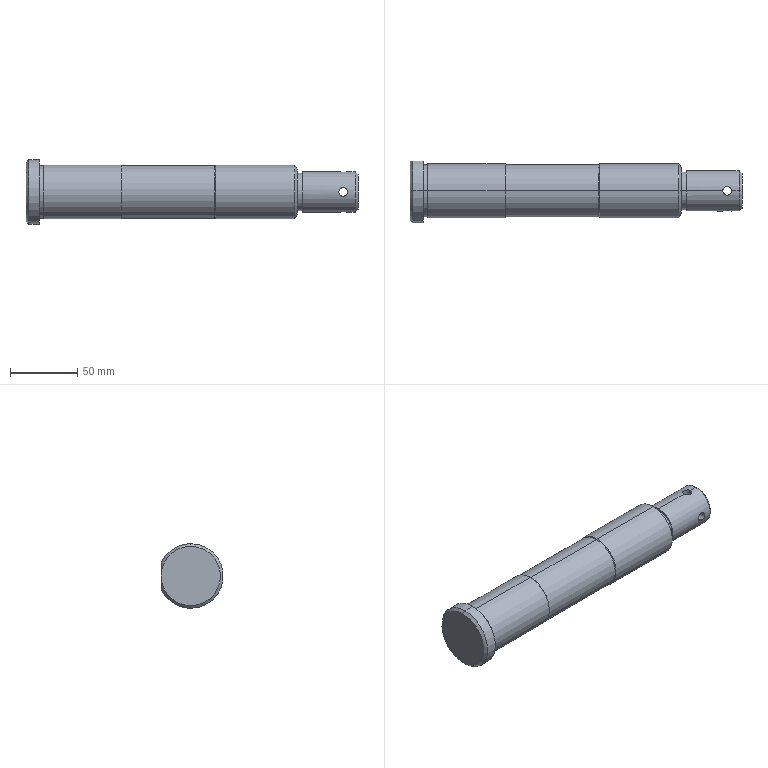Part | SolidWorks | features Chamfer 4, ICE 3, Revolution 1 | 1 solid | 41 faces | box 246 x 46 x 48 mm | volume 282253 mm3 | cylinder 23 | cone 11 | plane 7 | commonest cylinder face diameters 6.5 x8 39 x4 40 x4 48 x3 28 x2 30 x2